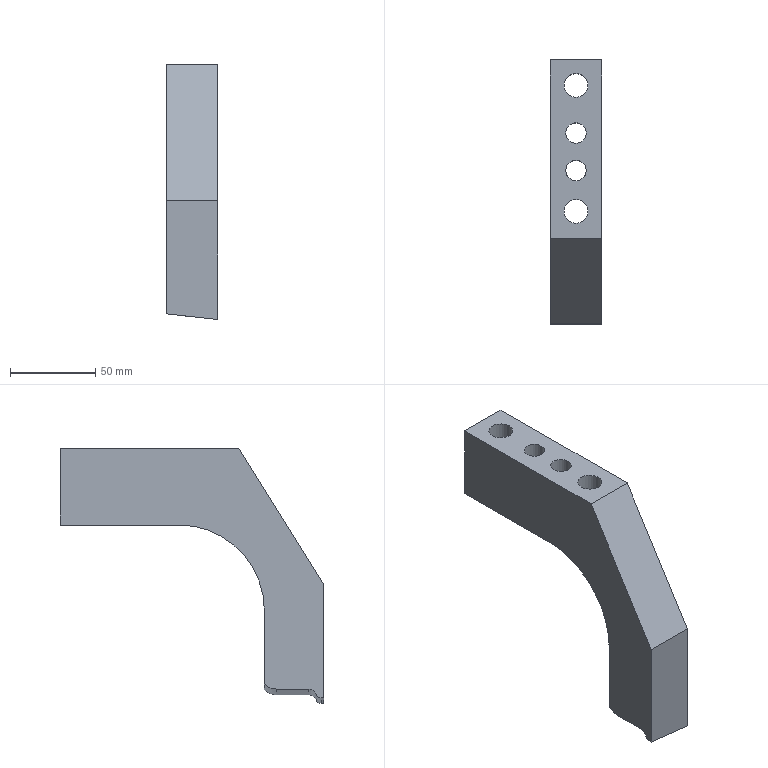Part | NX | features solid 2 | 1 solid | 23 faces | box 30 x 155 x 149.883 mm | volume 237197 mm3 | plane 9 | cylinder 7 | spline 7 | commonest cylinder face diameters 12 x2 14 x2 20 x2 100 x1
STEP:
#1=CARTESIAN_POINT('',(-215.,-438.,-38.417));
#2=VERTEX_POINT('',#1);
#3=CARTESIAN_POINT('',(-185.,-438.,-41.703));
#4=VERTEX_POINT('',#3);
#5=CARTESIAN_POINT('',(-215.,-438.,-38.417));
#6=CARTESIAN_POINT('',(-205.006,-438.,-39.569));
#7=CARTESIAN_POINT('',(-195.006,-438.,-40.665));
#8=CARTESIAN_POINT('',(-185.,-438.,-41.703));
#9=B_SPLINE_CURVE_WITH_KNOTS('',3,(#5,#6,#7,#8),.UNSPECIFIED.,.F.,.F.,(4,4),(0.,0.03018),.UNSPECIFIED.);
#10=EDGE_CURVE('',#2,#4,#9,.T.);
#11=ORIENTED_EDGE('',*,*,#10,.F.);
#12=CARTESIAN_POINT('',(-215.,-438.,5.));
#13=VERTEX_POINT('',#12);
#14=CARTESIAN_POINT('',(-215.,-438.,-220.));
#15=DIRECTION('',(0.,0.,-1.));
#16=VECTOR('',#15,1000.);
#17=LINE('',#14,#16);
#18=EDGE_CURVE('',#13,#2,#17,.T.);
#19=ORIENTED_EDGE('',*,*,#18,.F.);
#20=CARTESIAN_POINT('',(-185.,-438.,5.));
#21=VERTEX_POINT('',#20);
#22=CARTESIAN_POINT('',(-200.,-438.,5.));
#23=DIRECTION('',(-1.,0.,0.));
#24=VECTOR('',#23,1000.);
#25=LINE('',#22,#24);
#26=EDGE_CURVE('',#13,#21,#25,.F.);
#27=ORIENTED_EDGE('',*,*,#26,.T.);
#28=CARTESIAN_POINT('',(-185.,-438.,55.));
#29=DIRECTION('',(0.,0.,-1.));
#30=VECTOR('',#29,1000.);
#31=LINE('',#28,#30);
#32=EDGE_CURVE('',#21,#4,#31,.T.);
#33=ORIENTED_EDGE('',*,*,#32,.T.);
#34=EDGE_LOOP('',(#11,#19,#27,#33));
#35=FACE_BOUND('',#34,.T.);
#36=CARTESIAN_POINT('',(-200.,-438.,17.572));
#37=DIRECTION('',(0.,-1.,0.));
#38=DIRECTION('',(0.,0.,-1.));
#39=AXIS2_PLACEMENT_3D('',#36,#37,#38);
#40=PLANE('',#39);
#41=ADVANCED_FACE('',(#35),#40,.F.);
#42=CARTESIAN_POINT('',(-215.,-473.,20.));
#43=VERTEX_POINT('',#42);
#44=CARTESIAN_POINT('',(-215.,-473.,-46.541));
#45=VERTEX_POINT('',#44);
#46=CARTESIAN_POINT('',(-215.,-473.,-220.));
#47=DIRECTION('',(0.,0.,-1.));
#48=VECTOR('',#47,1000.);
#49=LINE('',#46,#48);
#50=EDGE_CURVE('',#43,#45,#49,.T.);
#51=ORIENTED_EDGE('',*,*,#50,.F.);
#52=CARTESIAN_POINT('',(-215.,-423.,100.));
#53=VERTEX_POINT('',#52);
#54=CARTESIAN_POINT('',(-215.,-423.,100.));
#55=DIRECTION('',(0.,0.53,0.848));
#56=VECTOR('',#55,1000.);
#57=LINE('',#54,#56);
#58=EDGE_CURVE('',#43,#53,#57,.T.);
#59=ORIENTED_EDGE('',*,*,#58,.T.);
#60=CARTESIAN_POINT('',(-215.,-318.,100.));
#61=VERTEX_POINT('',#60);
#62=CARTESIAN_POINT('',(-215.,-449.718,100.));
#63=DIRECTION('',(0.,1.,0.));
#64=VECTOR('',#63,1000.);
#65=LINE('',#62,#64);
#66=EDGE_CURVE('',#53,#61,#65,.T.);
#67=ORIENTED_EDGE('',*,*,#66,.T.);
#68=CARTESIAN_POINT('',(-215.,-318.,55.));
#69=VERTEX_POINT('',#68);
#70=CARTESIAN_POINT('',(-215.,-318.,-220.));
#71=DIRECTION('',(0.,0.,-1.));
#72=VECTOR('',#71,1000.);
#73=LINE('',#70,#72);
#74=EDGE_CURVE('',#61,#69,#73,.T.);
#75=ORIENTED_EDGE('',*,*,#74,.T.);
#76=CARTESIAN_POINT('',(-215.,-388.,55.));
#77=VERTEX_POINT('',#76);
#78=CARTESIAN_POINT('',(-215.,-449.718,55.));
#79=DIRECTION('',(0.,-1.,0.));
#80=VECTOR('',#79,1000.);
#81=LINE('',#78,#80);
#82=EDGE_CURVE('',#69,#77,#81,.T.);
#83=ORIENTED_EDGE('',*,*,#82,.T.);
#84=CARTESIAN_POINT('',(-215.,-388.,5.));
#85=DIRECTION('',(1.,0.,0.));
#86=DIRECTION('',(0.,0.,-1.));
#87=AXIS2_PLACEMENT_3D('',#84,#85,#86);
#88=CIRCLE('',#87,50.);
#89=EDGE_CURVE('',#77,#13,#88,.T.);
#90=ORIENTED_EDGE('',*,*,#89,.T.);
#91=ORIENTED_EDGE('',*,*,#18,.T.);
#92=CARTESIAN_POINT('',(-215.,-445.117,-41.44));
#93=VERTEX_POINT('',#92);
#94=CARTESIAN_POINT('',(-215.,-445.12,-41.44));
#95=CARTESIAN_POINT('',(-215.,-442.447,-41.433));
#96=CARTESIAN_POINT('',(-215.,-439.84,-40.307));
#97=CARTESIAN_POINT('',(-215.,-438.,-38.417));
#98=B_SPLINE_CURVE_WITH_KNOTS('',3,(#94,#95,#96,#97),.UNSPECIFIED.,.F.,.F.,(4,4),(0.,0.007904),.UNSPECIFIED.);
#99=EDGE_CURVE('',#93,#2,#98,.T.);
#100=ORIENTED_EDGE('',*,*,#99,.F.);
#101=CARTESIAN_POINT('',(-215.,-464.023,-41.485));
#102=VERTEX_POINT('',#101);
#103=CARTESIAN_POINT('',(-215.,-445.11,-41.44));
#104=CARTESIAN_POINT('',(-215.,-451.414,-41.455));
#105=CARTESIAN_POINT('',(-215.,-457.718,-41.471));
#106=CARTESIAN_POINT('',(-215.,-464.023,-41.485));
#107=B_SPLINE_CURVE_WITH_KNOTS('',3,(#103,#104,#105,#106),.UNSPECIFIED.,.F.,.F.,(4,4),(0.01573,0.03464),.UNSPECIFIED.);
#108=EDGE_CURVE('',#93,#102,#107,.T.);
#109=ORIENTED_EDGE('',*,*,#108,.T.);
#110=CARTESIAN_POINT('',(-215.,-468.65,-44.642));
#111=VERTEX_POINT('',#110);
#112=CARTESIAN_POINT('',(-215.,-464.023,-41.485));
#113=CARTESIAN_POINT('',(-215.,-466.022,-41.49));
#114=CARTESIAN_POINT('',(-215.,-467.91,-42.787));
#115=CARTESIAN_POINT('',(-215.,-468.65,-44.643));
#116=B_SPLINE_CURVE_WITH_KNOTS('',3,(#112,#113,#114,#115),.UNSPECIFIED.,.F.,.F.,(4,4),(0.,0.005912),.UNSPECIFIED.);
#117=EDGE_CURVE('',#102,#111,#116,.T.);
#118=ORIENTED_EDGE('',*,*,#117,.T.);
#119=CARTESIAN_POINT('',(-215.,-471.426,-46.537));
#120=VERTEX_POINT('',#119);
#121=CARTESIAN_POINT('',(-215.,-471.424,-46.537));
#122=CARTESIAN_POINT('',(-215.,-470.825,-46.534));
#123=CARTESIAN_POINT('',(-215.,-469.586,-46.252));
#124=CARTESIAN_POINT('',(-215.,-468.869,-45.194));
#125=CARTESIAN_POINT('',(-215.,-468.649,-44.64));
#126=B_SPLINE_CURVE_WITH_KNOTS('',3,(#121,#122,#123,#124,#125),.UNSPECIFIED.,.F.,.F.,(4,1,4),(0.001591,0.003375,0.00516),.UNSPECIFIED.);
#127=EDGE_CURVE('',#120,#111,#126,.T.);
#128=ORIENTED_EDGE('',*,*,#127,.F.);
#129=CARTESIAN_POINT('',(-215.,-471.431,-46.537));
#130=CARTESIAN_POINT('',(-215.,-471.954,-46.538));
#131=CARTESIAN_POINT('',(-215.,-472.477,-46.54));
#132=CARTESIAN_POINT('',(-215.,-473.,-46.541));
#133=B_SPLINE_CURVE_WITH_KNOTS('',3,(#129,#130,#131,#132),.UNSPECIFIED.,.F.,.F.,(4,4),(0.005963,0.007533),.UNSPECIFIED.);
#134=EDGE_CURVE('',#120,#45,#133,.T.);
#135=ORIENTED_EDGE('',*,*,#134,.T.);
#136=EDGE_LOOP('',(#51,#59,#67,#75,#83,#90,#91,#100,#109,#118,#128,#135));
#137=FACE_BOUND('',#136,.T.);
#138=CARTESIAN_POINT('',(-215.,-449.718,-220.));
#139=DIRECTION('',(1.,0.,0.));
#140=DIRECTION('',(0.,0.,-1.));
#141=AXIS2_PLACEMENT_3D('',#138,#139,#140);
#142=PLANE('',#141);
#143=ADVANCED_FACE('',(#137),#142,.F.);
#144=CARTESIAN_POINT('',(-185.,-423.,100.));
#145=VERTEX_POINT('',#144);
#146=CARTESIAN_POINT('',(-185.,-318.,100.));
#147=VERTEX_POINT('',#146);
#148=CARTESIAN_POINT('',(-185.,-425.,100.));
#149=DIRECTION('',(0.,1.,0.));
#150=VECTOR('',#149,1000.);
#151=LINE('',#148,#150);
#152=EDGE_CURVE('',#145,#147,#151,.T.);
#153=ORIENTED_EDGE('',*,*,#152,.F.);
#154=CARTESIAN_POINT('',(-185.,-473.,20.));
#155=VERTEX_POINT('',#154);
#156=CARTESIAN_POINT('',(-185.,-443.787,66.742));
#157=DIRECTION('',(0.,-0.53,-0.848));
#158=VECTOR('',#157,1000.);
#159=LINE('',#156,#158);
#160=EDGE_CURVE('',#145,#155,#159,.T.);
#161=ORIENTED_EDGE('',*,*,#160,.T.);
#162=CARTESIAN_POINT('',(-185.,-473.,-49.883));
#163=VERTEX_POINT('',#162);
#164=CARTESIAN_POINT('',(-185.,-473.,55.));
#165=DIRECTION('',(0.,0.,-1.));
#166=VECTOR('',#165,1000.);
#167=LINE('',#164,#166);
#168=EDGE_CURVE('',#155,#163,#167,.T.);
#169=ORIENTED_EDGE('',*,*,#168,.T.);
#170=CARTESIAN_POINT('',(-185.,-471.426,-49.879));
#171=VERTEX_POINT('',#170);
#172=CARTESIAN_POINT('',(-185.,-471.43,-49.88));
#173=CARTESIAN_POINT('',(-185.,-471.953,-49.881));
#174=CARTESIAN_POINT('',(-185.,-472.477,-49.882));
#175=CARTESIAN_POINT('',(-185.,-473.,-49.883));
#176=B_SPLINE_CURVE_WITH_KNOTS('',3,(#172,#173,#174,#175),.UNSPECIFIED.,.F.,.F.,(4,4),(0.005972,0.007542),.UNSPECIFIED.);
#177=EDGE_CURVE('',#171,#163,#176,.T.);
#178=ORIENTED_EDGE('',*,*,#177,.F.);
#179=CARTESIAN_POINT('',(-185.,-468.65,-47.987));
#180=VERTEX_POINT('',#179);
#181=CARTESIAN_POINT('',(-185.,-471.425,-49.879));
#182=CARTESIAN_POINT('',(-185.,-470.826,-49.876));
#183=CARTESIAN_POINT('',(-185.,-469.588,-49.596));
#184=CARTESIAN_POINT('',(-185.,-468.87,-48.54));
#185=CARTESIAN_POINT('',(-185.,-468.649,-47.986));
#186=B_SPLINE_CURVE_WITH_KNOTS('',3,(#181,#182,#183,#184,#185),.UNSPECIFIED.,.F.,.F.,(4,1,4),(0.00159,0.003374,0.005157),.UNSPECIFIED.);
#187=EDGE_CURVE('',#171,#180,#186,.T.);
#188=ORIENTED_EDGE('',*,*,#187,.T.);
#189=CARTESIAN_POINT('',(-185.,-464.023,-44.835));
#190=VERTEX_POINT('',#189);
#191=CARTESIAN_POINT('',(-185.,-464.023,-44.835));
#192=CARTESIAN_POINT('',(-185.,-466.021,-44.839));
#193=CARTESIAN_POINT('',(-185.,-467.91,-46.134));
#194=CARTESIAN_POINT('',(-185.,-468.65,-47.988));
#195=B_SPLINE_CURVE_WITH_KNOTS('',3,(#191,#192,#193,#194),.UNSPECIFIED.,.F.,.F.,(4,4),(0.,0.005909),.UNSPECIFIED.);
#196=EDGE_CURVE('',#190,#180,#195,.T.);
#197=ORIENTED_EDGE('',*,*,#196,.F.);
#198=CARTESIAN_POINT('',(-185.,-445.183,-44.789));
#199=VERTEX_POINT('',#198);
#200=CARTESIAN_POINT('',(-185.,-445.176,-44.789));
#201=CARTESIAN_POINT('',(-185.,-451.458,-44.805));
#202=CARTESIAN_POINT('',(-185.,-457.74,-44.82));
#203=CARTESIAN_POINT('',(-185.,-464.023,-44.835));
#204=B_SPLINE_CURVE_WITH_KNOTS('',3,(#200,#201,#202,#203),.UNSPECIFIED.,.F.,.F.,(4,4),(0.0158,0.03465),.UNSPECIFIED.);
#205=EDGE_CURVE('',#199,#190,#204,.T.);
#206=ORIENTED_EDGE('',*,*,#205,.F.);
#207=CARTESIAN_POINT('',(-185.,-445.185,-44.789));
#208=CARTESIAN_POINT('',(-185.,-442.481,-44.783));
#209=CARTESIAN_POINT('',(-185.,-439.843,-43.631));
#210=CARTESIAN_POINT('',(-185.,-438.,-41.703));
#211=B_SPLINE_CURVE_WITH_KNOTS('',3,(#207,#208,#209,#210),.UNSPECIFIED.,.F.,.F.,(4,4),(0.,0.007995),.UNSPECIFIED.);
#212=EDGE_CURVE('',#199,#4,#211,.T.);
#213=ORIENTED_EDGE('',*,*,#212,.T.);
#214=ORIENTED_EDGE('',*,*,#32,.F.);
#215=CARTESIAN_POINT('',(-185.,-388.,55.));
#216=VERTEX_POINT('',#215);
#217=CARTESIAN_POINT('',(-185.,-388.,5.));
#218=DIRECTION('',(1.,0.,0.));
#219=DIRECTION('',(0.,0.,-1.));
#220=AXIS2_PLACEMENT_3D('',#217,#218,#219);
#221=CIRCLE('',#220,50.);
#222=EDGE_CURVE('',#21,#216,#221,.F.);
#223=ORIENTED_EDGE('',*,*,#222,.T.);
#224=CARTESIAN_POINT('',(-185.,-318.,55.));
#225=VERTEX_POINT('',#224);
#226=CARTESIAN_POINT('',(-185.,-425.,55.));
#227=DIRECTION('',(0.,1.,0.));
#228=VECTOR('',#227,1000.);
#229=LINE('',#226,#228);
#230=EDGE_CURVE('',#216,#225,#229,.T.);
#231=ORIENTED_EDGE('',*,*,#230,.T.);
#232=CARTESIAN_POINT('',(-185.,-318.,55.));
#233=DIRECTION('',(0.,0.,-1.));
#234=VECTOR('',#233,1000.);
#235=LINE('',#232,#234);
#236=EDGE_CURVE('',#147,#225,#235,.T.);
#237=ORIENTED_EDGE('',*,*,#236,.F.);
#238=EDGE_LOOP('',(#153,#161,#169,#178,#188,#197,#206,#213,#214,#223,#231,#237));
#239=FACE_BOUND('',#238,.T.);
#240=CARTESIAN_POINT('',(-185.,-425.,55.));
#241=DIRECTION('',(1.,0.,0.));
#242=DIRECTION('',(0.,0.,-1.));
#243=AXIS2_PLACEMENT_3D('',#240,#241,#242);
#244=PLANE('',#243);
#245=ADVANCED_FACE('',(#239),#244,.T.);
#246=CARTESIAN_POINT('',(-207.,-333.,100.));
#247=VERTEX_POINT('',#246);
#248=CARTESIAN_POINT('',(-200.,-333.,100.));
#249=DIRECTION('',(0.,0.,-1.));
#250=DIRECTION('',(-1.,0.,0.));
#251=AXIS2_PLACEMENT_3D('',#248,#249,#250);
#252=CIRCLE('',#251,7.);
#253=EDGE_CURVE('',#247,#247,#252,.T.);
#254=ORIENTED_EDGE('',*,*,#253,.T.);
#255=EDGE_LOOP('',(#254));
#256=FACE_BOUND('',#255,.T.);
#257=CARTESIAN_POINT('',(-207.,-407.,100.));
#258=VERTEX_POINT('',#257);
#259=CARTESIAN_POINT('',(-200.,-407.,100.));
#260=DIRECTION('',(0.,0.,-1.));
#261=DIRECTION('',(-1.,0.,0.));
#262=AXIS2_PLACEMENT_3D('',#259,#260,#261);
#263=CIRCLE('',#262,7.);
#264=EDGE_CURVE('',#258,#258,#263,.T.);
#265=ORIENTED_EDGE('',*,*,#264,.T.);
#266=EDGE_LOOP('',(#265));
#267=FACE_BOUND('',#266,.T.);
#268=CARTESIAN_POINT('',(-206.,-361.,100.));
#269=VERTEX_POINT('',#268);
#270=CARTESIAN_POINT('',(-200.,-361.,100.));
#271=DIRECTION('',(0.,0.,-1.));
#272=DIRECTION('',(-1.,0.,0.));
#273=AXIS2_PLACEMENT_3D('',#270,#271,#272);
#274=CIRCLE('',#273,6.);
#275=EDGE_CURVE('',#269,#269,#274,.T.);
#276=ORIENTED_EDGE('',*,*,#275,.T.);
#277=EDGE_LOOP('',(#276));
#278=FACE_BOUND('',#277,.T.);
#279=CARTESIAN_POINT('',(-206.,-383.,100.));
#280=VERTEX_POINT('',#279);
#281=CARTESIAN_POINT('',(-200.,-383.,100.));
#282=DIRECTION('',(0.,0.,-1.));
#283=DIRECTION('',(-1.,0.,0.));
#284=AXIS2_PLACEMENT_3D('',#281,#282,#283);
#285=CIRCLE('',#284,6.);
#286=EDGE_CURVE('',#280,#280,#285,.T.);
#287=ORIENTED_EDGE('',*,*,#286,.T.);
#288=EDGE_LOOP('',(#287));
#289=FACE_BOUND('',#288,.T.);
#290=ORIENTED_EDGE('',*,*,#66,.F.);
#291=CARTESIAN_POINT('',(-185.,-423.,100.));
#292=DIRECTION('',(1.,0.,0.));
#293=VECTOR('',#292,1000.);
#294=LINE('',#291,#293);
#295=EDGE_CURVE('',#53,#145,#294,.T.);
#296=ORIENTED_EDGE('',*,*,#295,.T.);
#297=ORIENTED_EDGE('',*,*,#152,.T.);
#298=CARTESIAN_POINT('',(-255.,-318.,100.));
#299=DIRECTION('',(-1.,0.,0.));
#300=VECTOR('',#299,1000.);
#301=LINE('',#298,#300);
#302=EDGE_CURVE('',#147,#61,#301,.T.);
#303=ORIENTED_EDGE('',*,*,#302,.T.);
#304=EDGE_LOOP('',(#290,#296,#297,#303));
#305=FACE_BOUND('',#304,.T.);
#306=CARTESIAN_POINT('',(-255.,-425.,100.));
#307=DIRECTION('',(0.,0.,-1.));
#308=DIRECTION('',(-1.,0.,0.));
#309=AXIS2_PLACEMENT_3D('',#306,#307,#308);
#310=PLANE('',#309);
#311=ADVANCED_FACE('',(#256,#267,#278,#289,#305),#310,.F.);
#312=CARTESIAN_POINT('',(-190.,-333.,75.));
#313=VERTEX_POINT('',#312);
#314=CARTESIAN_POINT('',(-200.,-333.,75.));
#315=DIRECTION('',(0.,0.,-1.));
#316=DIRECTION('',(1.,0.,0.));
#317=AXIS2_PLACEMENT_3D('',#314,#315,#316);
#318=CIRCLE('',#317,10.);
#319=EDGE_CURVE('',#313,#313,#318,.T.);
#320=ORIENTED_EDGE('',*,*,#319,.F.);
#321=EDGE_LOOP('',(#320));
#322=FACE_BOUND('',#321,.T.);
#323=CARTESIAN_POINT('',(-210.,-333.,55.));
#324=VERTEX_POINT('',#323);
#325=CARTESIAN_POINT('',(-200.,-333.,55.));
#326=DIRECTION('',(0.,0.,-1.));
#327=DIRECTION('',(-1.,0.,0.));
#328=AXIS2_PLACEMENT_3D('',#325,#326,#327);
#329=CIRCLE('',#328,10.);
#330=EDGE_CURVE('',#324,#324,#329,.F.);
#331=ORIENTED_EDGE('',*,*,#330,.F.);
#332=EDGE_LOOP('',(#331));
#333=FACE_BOUND('',#332,.T.);
#334=CARTESIAN_POINT('',(-200.,-333.,75.));
#335=DIRECTION('',(0.,0.,-1.));
#336=DIRECTION('',(1.,0.,0.));
#337=AXIS2_PLACEMENT_3D('',#334,#335,#336);
#338=CYLINDRICAL_SURFACE('',#337,10.);
#339=ADVANCED_FACE('',(#322,#333),#338,.F.);
#340=CARTESIAN_POINT('',(-196.683,-397.566,54.076));
#341=VERTEX_POINT('',#340);
#342=CARTESIAN_POINT('',(-203.317,-397.566,54.076));
#343=VERTEX_POINT('',#342);
#344=CARTESIAN_POINT('',(-196.683,-397.566,54.076));
#345=CARTESIAN_POINT('',(-198.827,-396.813,54.223));
#346=CARTESIAN_POINT('',(-201.178,-396.814,54.223));
#347=CARTESIAN_POINT('',(-203.317,-397.566,54.076));
#348=B_SPLINE_CURVE_WITH_KNOTS('',3,(#344,#345,#346,#347),.UNSPECIFIED.,.F.,.F.,(4,4),(0.00252,0.009295),.UNSPECIFIED.);
#349=EDGE_CURVE('',#341,#343,#348,.T.);
#350=ORIENTED_EDGE('',*,*,#349,.F.);
#351=CARTESIAN_POINT('',(-196.683,-397.566,54.076));
#352=CARTESIAN_POINT('',(-194.359,-398.383,53.917));
#353=CARTESIAN_POINT('',(-190.433,-401.807,53.222));
#354=CARTESIAN_POINT('',(-189.595,-407.87,51.002));
#355=CARTESIAN_POINT('',(-191.169,-412.07,48.866));
#356=CARTESIAN_POINT('',(-193.31,-414.69,47.309));
#357=CARTESIAN_POINT('',(-196.321,-416.532,46.069));
#358=CARTESIAN_POINT('',(-200.012,-417.236,45.56));
#359=CARTESIAN_POINT('',(-203.706,-416.522,46.076));
#360=CARTESIAN_POINT('',(-207.707,-414.057,47.736));
#361=CARTESIAN_POINT('',(-210.569,-409.042,50.578));
#362=CARTESIAN_POINT('',(-209.564,-401.814,53.218));
#363=CARTESIAN_POINT('',(-205.645,-398.384,53.917));
#364=CARTESIAN_POINT('',(-203.317,-397.566,54.076));
#365=B_SPLINE_CURVE_WITH_KNOTS('',3,(#351,#352,#353,#354,#355,#356,#357,#358,#359,#360,#361,#362,#363,#364),.UNSPECIFIED.,.F.,.F.,(4,1,1,1,1,1,1,1,1,1,1,4),(0.03954,0.04689,0.05424,0.05791,0.06159,0.06526,0.06894,0.07261,0.07629,0.08363,0.09098,0.09833),.UNSPECIFIED.);
#366=EDGE_CURVE('',#341,#343,#365,.T.);
#367=ORIENTED_EDGE('',*,*,#366,.T.);
#368=EDGE_LOOP('',(#350,#367));
#369=FACE_BOUND('',#368,.T.);
#370=CARTESIAN_POINT('',(-190.,-407.,75.));
#371=VERTEX_POINT('',#370);
#372=CARTESIAN_POINT('',(-200.,-407.,75.));
#373=DIRECTION('',(0.,0.,-1.));
#374=DIRECTION('',(1.,0.,0.));
#375=AXIS2_PLACEMENT_3D('',#372,#373,#374);
#376=CIRCLE('',#375,10.);
#377=EDGE_CURVE('',#371,#371,#376,.T.);
#378=ORIENTED_EDGE('',*,*,#377,.F.);
#379=EDGE_LOOP('',(#378));
#380=FACE_BOUND('',#379,.T.);
#381=CARTESIAN_POINT('',(-200.,-407.,75.));
#382=DIRECTION('',(0.,0.,-1.));
#383=DIRECTION('',(1.,0.,0.));
#384=AXIS2_PLACEMENT_3D('',#381,#382,#383);
#385=CYLINDRICAL_SURFACE('',#384,10.);
#386=ADVANCED_FACE('',(#369,#380),#385,.F.);
#387=ORIENTED_EDGE('',*,*,#275,.F.);
#388=EDGE_LOOP('',(#387));
#389=FACE_BOUND('',#388,.T.);
#390=CARTESIAN_POINT('',(-206.,-361.,55.));
#391=VERTEX_POINT('',#390);
#392=CARTESIAN_POINT('',(-200.,-361.,55.));
#393=DIRECTION('',(0.,0.,-1.));
#394=DIRECTION('',(-1.,0.,0.));
#395=AXIS2_PLACEMENT_3D('',#392,#393,#394);
#396=CIRCLE('',#395,6.);
#397=EDGE_CURVE('',#391,#391,#396,.T.);
#398=ORIENTED_EDGE('',*,*,#397,.T.);
#399=EDGE_LOOP('',(#398));
#400=FACE_BOUND('',#399,.T.);
#401=CARTESIAN_POINT('',(-200.,-361.,105.));
#402=DIRECTION('',(0.,0.,-1.));
#403=DIRECTION('',(-1.,0.,0.));
#404=AXIS2_PLACEMENT_3D('',#401,#402,#403);
#405=CYLINDRICAL_SURFACE('',#404,6.);
#406=ADVANCED_FACE('',(#389,#400),#405,.F.);
#407=ORIENTED_EDGE('',*,*,#286,.F.);
#408=EDGE_LOOP('',(#407));
#409=FACE_BOUND('',#408,.T.);
#410=CARTESIAN_POINT('',(-196.683,-388.,55.));
#411=VERTEX_POINT('',#410);
#412=CARTESIAN_POINT('',(-203.317,-388.,55.));
#413=VERTEX_POINT('',#412);
#414=CARTESIAN_POINT('',(-200.,-383.,55.));
#415=DIRECTION('',(0.,0.,-1.));
#416=DIRECTION('',(-1.,0.,0.));
#417=AXIS2_PLACEMENT_3D('',#414,#415,#416);
#418=CIRCLE('',#417,6.);
#419=EDGE_CURVE('',#411,#413,#418,.T.);
#420=ORIENTED_EDGE('',*,*,#419,.T.);
#421=CARTESIAN_POINT('',(-200.,-383.,55.));
#422=DIRECTION('',(0.,0.,-1.));
#423=DIRECTION('',(-1.,0.,0.));
#424=AXIS2_PLACEMENT_3D('',#421,#422,#423);
#425=CIRCLE('',#424,6.);
#426=EDGE_CURVE('',#413,#411,#425,.T.);
#427=ORIENTED_EDGE('',*,*,#426,.T.);
#428=EDGE_LOOP('',(#420,#427));
#429=FACE_BOUND('',#428,.T.);
#430=CARTESIAN_POINT('',(-200.,-383.,105.));
#431=DIRECTION('',(0.,0.,-1.));
#432=DIRECTION('',(-1.,0.,0.));
#433=AXIS2_PLACEMENT_3D('',#430,#431,#432);
#434=CYLINDRICAL_SURFACE('',#433,6.);
#435=ADVANCED_FACE('',(#409,#429),#434,.F.);
#436=CARTESIAN_POINT('',(-193.,-333.,75.));
#437=VERTEX_POINT('',#436);
#438=CARTESIAN_POINT('',(-200.,-333.,75.));
#439=DIRECTION('',(0.,0.,1.));
#440=DIRECTION('',(1.,0.,0.));
#441=AXIS2_PLACEMENT_3D('',#438,#439,#440);
#442=CIRCLE('',#441,7.);
#443=EDGE_CURVE('',#437,#437,#442,.T.);
#444=ORIENTED_EDGE('',*,*,#443,.F.);
#445=EDGE_LOOP('',(#444));
#446=FACE_BOUND('',#445,.T.);
#447=ORIENTED_EDGE('',*,*,#253,.F.);
#448=EDGE_LOOP('',(#447));
#449=FACE_BOUND('',#448,.T.);
#450=CARTESIAN_POINT('',(-200.,-333.,75.));
#451=DIRECTION('',(0.,0.,1.));
#452=DIRECTION('',(-1.,0.,0.));
#453=AXIS2_PLACEMENT_3D('',#450,#451,#452);
#454=CYLINDRICAL_SURFACE('',#453,7.);
#455=ADVANCED_FACE('',(#446,#449),#454,.F.);
#456=ORIENTED_EDGE('',*,*,#443,.T.);
#457=EDGE_LOOP('',(#456));
#458=FACE_BOUND('',#457,.T.);
#459=ORIENTED_EDGE('',*,*,#319,.T.);
#460=EDGE_LOOP('',(#459));
#461=FACE_BOUND('',#460,.T.);
#462=CARTESIAN_POINT('',(-200.,-333.,75.));
#463=DIRECTION('',(0.,0.,1.));
#464=DIRECTION('',(-1.,0.,0.));
#465=AXIS2_PLACEMENT_3D('',#462,#463,#464);
#466=PLANE('',#465);
#467=ADVANCED_FACE('',(#458,#461),#466,.F.);
#468=CARTESIAN_POINT('',(-193.,-407.,75.));
#469=VERTEX_POINT('',#468);
#470=CARTESIAN_POINT('',(-200.,-407.,75.));
#471=DIRECTION('',(0.,0.,1.));
#472=DIRECTION('',(1.,0.,0.));
#473=AXIS2_PLACEMENT_3D('',#470,#471,#472);
#474=CIRCLE('',#473,7.);
#475=EDGE_CURVE('',#469,#469,#474,.T.);
#476=ORIENTED_EDGE('',*,*,#475,.F.);
#477=EDGE_LOOP('',(#476));
#478=FACE_BOUND('',#477,.T.);
#479=ORIENTED_EDGE('',*,*,#264,.F.);
#480=EDGE_LOOP('',(#479));
#481=FACE_BOUND('',#480,.T.);
#482=CARTESIAN_POINT('',(-200.,-407.,75.));
#483=DIRECTION('',(0.,0.,1.));
#484=DIRECTION('',(-1.,0.,0.));
#485=AXIS2_PLACEMENT_3D('',#482,#483,#484);
#486=CYLINDRICAL_SURFACE('',#485,7.);
#487=ADVANCED_FACE('',(#478,#481),#486,.F.);
#488=ORIENTED_EDGE('',*,*,#475,.T.);
#489=EDGE_LOOP('',(#488));
#490=FACE_BOUND('',#489,.T.);
#491=ORIENTED_EDGE('',*,*,#377,.T.);
#492=EDGE_LOOP('',(#491));
#493=FACE_BOUND('',#492,.T.);
#494=CARTESIAN_POINT('',(-200.,-402.,75.));
#495=DIRECTION('',(0.,0.,1.));
#496=DIRECTION('',(-1.,0.,0.));
#497=AXIS2_PLACEMENT_3D('',#494,#495,#496);
#498=PLANE('',#497);
#499=ADVANCED_FACE('',(#490,#493),#498,.F.);
#500=ORIENTED_EDGE('',*,*,#230,.F.);
#501=CARTESIAN_POINT('',(-185.,-388.,55.));
#502=DIRECTION('',(-1.,0.,0.));
#503=VECTOR('',#502,1000.);
#504=LINE('',#501,#503);
#505=EDGE_CURVE('',#216,#411,#504,.T.);
#506=ORIENTED_EDGE('',*,*,#505,.T.);
#507=ORIENTED_EDGE('',*,*,#426,.F.);
#508=CARTESIAN_POINT('',(-185.,-388.,55.));
#509=DIRECTION('',(-1.,0.,0.));
#510=VECTOR('',#509,1000.);
#511=LINE('',#508,#510);
#512=EDGE_CURVE('',#413,#77,#511,.T.);
#513=ORIENTED_EDGE('',*,*,#512,.T.);
#514=ORIENTED_EDGE('',*,*,#82,.F.);
#515=CARTESIAN_POINT('',(-185.,-318.,55.));
#516=DIRECTION('',(-1.,0.,0.));
#517=VECTOR('',#516,1000.);
#518=LINE('',#515,#517);
#519=EDGE_CURVE('',#225,#69,#518,.T.);
#520=ORIENTED_EDGE('',*,*,#519,.F.);
#521=EDGE_LOOP('',(#500,#506,#507,#513,#514,#520));
#522=FACE_BOUND('',#521,.T.);
#523=ORIENTED_EDGE('',*,*,#397,.F.);
#524=EDGE_LOOP('',(#523));
#525=FACE_BOUND('',#524,.T.);
#526=ORIENTED_EDGE('',*,*,#330,.T.);
#527=EDGE_LOOP('',(#526));
#528=FACE_BOUND('',#527,.T.);
#529=CARTESIAN_POINT('',(-185.,-410.,55.));
#530=DIRECTION('',(0.,0.,-1.));
#531=DIRECTION('',(-1.,0.,0.));
#532=AXIS2_PLACEMENT_3D('',#529,#530,#531);
#533=PLANE('',#532);
#534=ADVANCED_FACE('',(#522,#525,#528),#533,.T.);
#535=ORIENTED_EDGE('',*,*,#236,.T.);
#536=ORIENTED_EDGE('',*,*,#519,.T.);
#537=ORIENTED_EDGE('',*,*,#74,.F.);
#538=ORIENTED_EDGE('',*,*,#302,.F.);
#539=EDGE_LOOP('',(#535,#536,#537,#538));
#540=FACE_BOUND('',#539,.T.);
#541=CARTESIAN_POINT('',(-215.,-318.,100.));
#542=CARTESIAN_POINT('',(-185.,-318.,100.));
#543=CARTESIAN_POINT('',(-215.,-318.,55.));
#544=CARTESIAN_POINT('',(-185.,-318.,55.));
#545=B_SPLINE_SURFACE_WITH_KNOTS('',1,1,((#541,#542),(#543,#544)),.PLANE_SURF.,.F.,.F.,.F.,(2,2),(2,2),(0.3333,0.4238),(0.3333,0.6667),.PIECEWISE_BEZIER_KNOTS.);
#546=ADVANCED_FACE('',(#540),#545,.F.);
#547=ORIENTED_EDGE('',*,*,#168,.F.);
#548=CARTESIAN_POINT('',(-215.,-473.,20.));
#549=DIRECTION('',(-1.,0.,0.));
#550=VECTOR('',#549,1000.);
#551=LINE('',#548,#550);
#552=EDGE_CURVE('',#155,#43,#551,.T.);
#553=ORIENTED_EDGE('',*,*,#552,.T.);
#554=ORIENTED_EDGE('',*,*,#50,.T.);
#555=CARTESIAN_POINT('',(-185.,-473.,-49.883));
#556=CARTESIAN_POINT('',(-195.007,-473.,-48.83));
#557=CARTESIAN_POINT('',(-205.007,-473.,-47.715));
#558=CARTESIAN_POINT('',(-215.,-473.,-46.541));
#559=B_SPLINE_CURVE_WITH_KNOTS('',3,(#555,#556,#557,#558),.UNSPECIFIED.,.F.,.F.,(4,4),(0.,0.03019),.UNSPECIFIED.);
#560=EDGE_CURVE('',#163,#45,#559,.T.);
#561=ORIENTED_EDGE('',*,*,#560,.F.);
#562=EDGE_LOOP('',(#547,#553,#554,#561));
#563=FACE_BOUND('',#562,.T.);
#564=CARTESIAN_POINT('',(-1500.,-473.,0.));
#565=DIRECTION('',(0.,-1.,0.));
#566=DIRECTION('',(0.,0.,-1.));
#567=AXIS2_PLACEMENT_3D('',#564,#565,#566);
#568=PLANE('',#567);
#569=ADVANCED_FACE('',(#563),#568,.T.);
#570=CARTESIAN_POINT('',(-196.683,-388.,5.));
#571=DIRECTION('',(1.,0.,0.));
#572=DIRECTION('',(0.,0.,-1.));
#573=AXIS2_PLACEMENT_3D('',#570,#571,#572);
#574=CIRCLE('',#573,50.);
#575=EDGE_CURVE('',#341,#411,#574,.F.);
#576=ORIENTED_EDGE('',*,*,#575,.F.);
#577=ORIENTED_EDGE('',*,*,#349,.T.);
#578=CARTESIAN_POINT('',(-203.317,-388.,5.));
#579=DIRECTION('',(-1.,0.,0.));
#580=DIRECTION('',(0.,0.,1.));
#581=AXIS2_PLACEMENT_3D('',#578,#579,#580);
#582=CIRCLE('',#581,50.);
#583=EDGE_CURVE('',#413,#343,#582,.F.);
#584=ORIENTED_EDGE('',*,*,#583,.F.);
#585=ORIENTED_EDGE('',*,*,#419,.F.);
#586=EDGE_LOOP('',(#576,#577,#584,#585));
#587=FACE_BOUND('',#586,.T.);
#588=CARTESIAN_POINT('',(-196.683,-388.,55.));
#589=CARTESIAN_POINT('',(-196.683,-392.857,55.));
#590=CARTESIAN_POINT('',(-196.683,-397.623,54.065));
#591=CARTESIAN_POINT('',(-197.067,-388.255,55.));
#592=CARTESIAN_POINT('',(-197.067,-393.098,54.975));
#593=CARTESIAN_POINT('',(-197.07,-397.846,54.022));
#594=CARTESIAN_POINT('',(-198.019,-388.763,55.));
#595=CARTESIAN_POINT('',(-198.019,-393.578,54.926));
#596=CARTESIAN_POINT('',(-198.025,-398.291,53.935));
#597=CARTESIAN_POINT('',(-200.,-389.119,55.));
#598=CARTESIAN_POINT('',(-200.,-393.914,54.893));
#599=CARTESIAN_POINT('',(-200.,-398.602,53.876));
#600=CARTESIAN_POINT('',(-201.981,-388.763,55.));
#601=CARTESIAN_POINT('',(-201.981,-393.578,54.926));
#602=CARTESIAN_POINT('',(-201.974,-398.291,53.935));
#603=CARTESIAN_POINT('',(-202.933,-388.255,55.));
#604=CARTESIAN_POINT('',(-202.933,-393.098,54.975));
#605=CARTESIAN_POINT('',(-202.93,-397.846,54.022));
#606=CARTESIAN_POINT('',(-203.317,-388.,55.));
#607=CARTESIAN_POINT('',(-203.317,-392.857,55.));
#608=CARTESIAN_POINT('',(-203.317,-397.623,54.065));
#609=(BOUNDED_SURFACE()B_SPLINE_SURFACE(3,2,((#588,#589,#590),(#591,#592,#593),(#594,#595,#596),(#597,#598,#599),(#600,#601,#602),(#603,#604,#605),(#606,#607,#608)),.UNSPECIFIED.,.F.,.F.,.F.)B_SPLINE_SURFACE_WITH_KNOTS((4,1,1,1,4),(3,3),(0.08051,0.08216,0.0838,0.08545,0.0871),(0.,0.1321),.UNSPECIFIED.)GEOMETRIC_REPRESENTATION_ITEM()RATIONAL_B_SPLINE_SURFACE(((1.,0.9613,0.9329),(1.,0.9616,0.9333),(1.,0.962,0.9341),(1.,0.9624,0.9347),(1.,0.962,0.9341),(1.,0.9616,0.9333),(1.,0.9613,0.9329)))REPRESENTATION_ITEM('')SURFACE());
#610=ADVANCED_FACE('',(#587),#609,.F.);
#611=ORIENTED_EDGE('',*,*,#222,.F.);
#612=ORIENTED_EDGE('',*,*,#26,.F.);
#613=ORIENTED_EDGE('',*,*,#89,.F.);
#614=ORIENTED_EDGE('',*,*,#512,.F.);
#615=ORIENTED_EDGE('',*,*,#583,.T.);
#616=ORIENTED_EDGE('',*,*,#366,.F.);
#617=ORIENTED_EDGE('',*,*,#575,.T.);
#618=ORIENTED_EDGE('',*,*,#505,.F.);
#619=EDGE_LOOP('',(#611,#612,#613,#614,#615,#616,#617,#618));
#620=FACE_BOUND('',#619,.T.);
#621=CARTESIAN_POINT('',(-185.,-388.,5.));
#622=DIRECTION('',(-1.,0.,0.));
#623=DIRECTION('',(0.,0.,1.));
#624=AXIS2_PLACEMENT_3D('',#621,#622,#623);
#625=CYLINDRICAL_SURFACE('',#624,50.);
#626=ADVANCED_FACE('',(#620),#625,.F.);
#627=ORIENTED_EDGE('',*,*,#127,.T.);
#628=CARTESIAN_POINT('',(-215.,-468.649,-44.64));
#629=CARTESIAN_POINT('',(-204.953,-468.649,-45.821));
#630=CARTESIAN_POINT('',(-194.953,-468.649,-46.937));
#631=CARTESIAN_POINT('',(-185.,-468.649,-47.986));
#632=B_SPLINE_CURVE_WITH_KNOTS('',3,(#628,#629,#630,#631),.UNSPECIFIED.,.F.,.F.,(4,4),(0.7825,0.8381),.UNSPECIFIED.);
#633=EDGE_CURVE('',#111,#180,#632,.T.);
#634=ORIENTED_EDGE('',*,*,#633,.T.);
#635=ORIENTED_EDGE('',*,*,#187,.F.);
#636=CARTESIAN_POINT('',(-185.,-471.425,-49.879));
#637=CARTESIAN_POINT('',(-194.953,-471.425,-48.831));
#638=CARTESIAN_POINT('',(-204.953,-471.424,-47.717));
#639=CARTESIAN_POINT('',(-215.,-471.424,-46.537));
#640=B_SPLINE_CURVE_WITH_KNOTS('',3,(#636,#637,#638,#639),.UNSPECIFIED.,.F.,.F.,(4,4),(0.1617,0.2174),.UNSPECIFIED.);
#641=EDGE_CURVE('',#171,#120,#640,.T.);
#642=ORIENTED_EDGE('',*,*,#641,.T.);
#643=EDGE_LOOP('',(#627,#634,#635,#642));
#644=FACE_BOUND('',#643,.T.);
#645=CARTESIAN_POINT('',(-184.799,-472.798,-49.73));
#646=CARTESIAN_POINT('',(-184.828,-471.841,-49.949));
#647=CARTESIAN_POINT('',(-184.83,-471.011,-49.99));
#648=CARTESIAN_POINT('',(-184.804,-470.308,-49.853));
#649=CARTESIAN_POINT('',(-184.732,-469.535,-49.433));
#650=CARTESIAN_POINT('',(-184.612,-468.983,-48.706));
#651=CARTESIAN_POINT('',(-184.578,-468.857,-48.5));
#652=CARTESIAN_POINT('',(-184.541,-468.744,-48.275));
#653=CARTESIAN_POINT('',(-184.501,-468.646,-48.03));
#654=CARTESIAN_POINT('',(-190.951,-472.469,-49.159));
#655=CARTESIAN_POINT('',(-190.973,-471.547,-49.329));
#656=CARTESIAN_POINT('',(-190.967,-470.752,-49.321));
#657=CARTESIAN_POINT('',(-190.934,-470.084,-49.136));
#658=CARTESIAN_POINT('',(-190.851,-469.358,-48.651));
#659=CARTESIAN_POINT('',(-190.721,-468.851,-47.861));
#660=CARTESIAN_POINT('',(-190.685,-468.736,-47.64));
#661=CARTESIAN_POINT('',(-190.645,-468.634,-47.399));
#662=CARTESIAN_POINT('',(-190.603,-468.547,-47.138));
#663=CARTESIAN_POINT('',(-197.096,-472.172,-48.544));
#664=CARTESIAN_POINT('',(-197.111,-471.282,-48.668));
#665=CARTESIAN_POINT('',(-197.098,-470.521,-48.614));
#666=CARTESIAN_POINT('',(-197.057,-469.887,-48.382));
#667=CARTESIAN_POINT('',(-196.965,-469.204,-47.837));
#668=CARTESIAN_POINT('',(-196.826,-468.739,-46.988));
#669=CARTESIAN_POINT('',(-196.787,-468.635,-46.751));
#670=CARTESIAN_POINT('',(-196.745,-468.544,-46.495));
#671=CARTESIAN_POINT('',(-196.7,-468.468,-46.22));
#672=CARTESIAN_POINT('',(-203.235,-471.902,-47.89));
#673=CARTESIAN_POINT('',(-203.243,-471.045,-47.969));
#674=CARTESIAN_POINT('',(-203.223,-470.315,-47.871));
#675=CARTESIAN_POINT('',(-203.176,-469.712,-47.597));
#676=CARTESIAN_POINT('',(-203.075,-469.07,-46.994));
#677=CARTESIAN_POINT('',(-202.927,-468.645,-46.089));
#678=CARTESIAN_POINT('',(-202.886,-468.551,-45.839));
#679=CARTESIAN_POINT('',(-202.842,-468.471,-45.569));
#680=CARTESIAN_POINT('',(-202.795,-468.404,-45.279));
#681=CARTESIAN_POINT('',(-209.369,-471.659,-47.2));
#682=CARTESIAN_POINT('',(-209.37,-470.831,-47.238));
#683=CARTESIAN_POINT('',(-209.344,-470.131,-47.099));
#684=CARTESIAN_POINT('',(-209.29,-469.557,-46.783));
#685=CARTESIAN_POINT('',(-209.18,-468.954,-46.127));
#686=CARTESIAN_POINT('',(-209.024,-468.567,-45.17));
#687=CARTESIAN_POINT('',(-208.981,-468.482,-44.906));
#688=CARTESIAN_POINT('',(-208.935,-468.411,-44.622));
#689=CARTESIAN_POINT('',(-208.886,-468.354,-44.32));
#690=CARTESIAN_POINT('',(-215.497,-471.438,-46.479));
#691=CARTESIAN_POINT('',(-215.493,-470.638,-46.477));
#692=CARTESIAN_POINT('',(-215.46,-469.966,-46.299));
#693=CARTESIAN_POINT('',(-215.4,-469.42,-45.945));
#694=CARTESIAN_POINT('',(-215.283,-468.852,-45.238));
#695=CARTESIAN_POINT('',(-215.119,-468.501,-44.232));
#696=CARTESIAN_POINT('',(-215.074,-468.425,-43.955));
#697=CARTESIAN_POINT('',(-215.026,-468.363,-43.66));
#698=CARTESIAN_POINT('',(-214.974,-468.315,-43.344));
#699=B_SPLINE_SURFACE_WITH_KNOTS('',5,5,((#645,#646,#647,#648,#649,#650,#651,#652,#653),(#654,#655,#656,#657,#658,#659,#660,#661,#662),(#663,#664,#665,#666,#667,#668,#669,#670,#671),(#672,#673,#674,#675,#676,#677,#678,#679,#680),(#681,#682,#683,#684,#685,#686,#687,#688,#689),(#690,#691,#692,#693,#694,#695,#696,#697,#698)),.UNSPECIFIED.,.F.,.F.,.F.,(6,6),(6,3,6),(0.1524,0.2052),(0.2588,0.486,0.5639),.UNSPECIFIED.);
#700=ADVANCED_FACE('',(#644),#699,.T.);
#701=CARTESIAN_POINT('',(-185.,-464.023,-44.835));
#702=CARTESIAN_POINT('',(-195.003,-464.023,-43.779));
#703=CARTESIAN_POINT('',(-205.003,-464.023,-42.662));
#704=CARTESIAN_POINT('',(-215.,-464.023,-41.485));
#705=B_SPLINE_CURVE_WITH_KNOTS('',3,(#701,#702,#703,#704),.UNSPECIFIED.,.F.,.F.,(4,4),(0.165,0.2227),.UNSPECIFIED.);
#706=EDGE_CURVE('',#190,#102,#705,.T.);
#707=ORIENTED_EDGE('',*,*,#706,.F.);
#708=ORIENTED_EDGE('',*,*,#196,.T.);
#709=ORIENTED_EDGE('',*,*,#633,.F.);
#710=ORIENTED_EDGE('',*,*,#117,.F.);
#711=EDGE_LOOP('',(#707,#708,#709,#710));
#712=FACE_BOUND('',#711,.T.);
#713=CARTESIAN_POINT('',(-184.489,-464.023,-44.888));
#714=CARTESIAN_POINT('',(-184.49,-465.209,-44.891));
#715=CARTESIAN_POINT('',(-184.527,-466.395,-45.244));
#716=CARTESIAN_POINT('',(-184.601,-467.439,-45.948));
#717=CARTESIAN_POINT('',(-184.702,-468.208,-46.912));
#718=CARTESIAN_POINT('',(-184.818,-468.65,-48.007));
#719=CARTESIAN_POINT('',(-190.63,-464.023,-44.242));
#720=CARTESIAN_POINT('',(-190.63,-465.209,-44.245));
#721=CARTESIAN_POINT('',(-190.668,-466.395,-44.597));
#722=CARTESIAN_POINT('',(-190.744,-467.439,-45.301));
#723=CARTESIAN_POINT('',(-190.848,-468.208,-46.265));
#724=CARTESIAN_POINT('',(-190.966,-468.65,-47.36));
#725=CARTESIAN_POINT('',(-196.769,-464.023,-43.576));
#726=CARTESIAN_POINT('',(-196.769,-465.209,-43.579));
#727=CARTESIAN_POINT('',(-196.808,-466.395,-43.931));
#728=CARTESIAN_POINT('',(-196.886,-467.439,-44.635));
#729=CARTESIAN_POINT('',(-196.992,-468.208,-45.599));
#730=CARTESIAN_POINT('',(-197.113,-468.65,-46.693));
#731=CARTESIAN_POINT('',(-202.907,-464.023,-42.891));
#732=CARTESIAN_POINT('',(-202.908,-465.209,-42.894));
#733=CARTESIAN_POINT('',(-202.947,-466.395,-43.246));
#734=CARTESIAN_POINT('',(-203.027,-467.439,-43.949));
#735=CARTESIAN_POINT('',(-203.136,-468.208,-44.913));
#736=CARTESIAN_POINT('',(-203.259,-468.65,-46.007));
#737=CARTESIAN_POINT('',(-209.045,-464.023,-42.187));
#738=CARTESIAN_POINT('',(-209.045,-465.209,-42.19));
#739=CARTESIAN_POINT('',(-209.086,-466.395,-42.542));
#740=CARTESIAN_POINT('',(-209.167,-467.439,-43.245));
#741=CARTESIAN_POINT('',(-209.278,-468.208,-44.208));
#742=CARTESIAN_POINT('',(-209.404,-468.65,-45.302));
#743=CARTESIAN_POINT('',(-215.182,-464.023,-41.464));
#744=CARTESIAN_POINT('',(-215.182,-465.209,-41.467));
#745=CARTESIAN_POINT('',(-215.224,-466.395,-41.819));
#746=CARTESIAN_POINT('',(-215.307,-467.439,-42.522));
#747=CARTESIAN_POINT('',(-215.42,-468.208,-43.485));
#748=CARTESIAN_POINT('',(-215.549,-468.65,-44.578));
#749=B_SPLINE_SURFACE_WITH_KNOTS('',5,5,((#713,#714,#715,#716,#717,#718),(#719,#720,#721,#722,#723,#724),(#725,#726,#727,#728,#729,#730),(#731,#732,#733,#734,#735,#736),(#737,#738,#739,#740,#741,#742),(#743,#744,#745,#746,#747,#748)),.UNSPECIFIED.,.F.,.F.,.F.,(6,6),(6,6),(0.1497,0.2036),(0.,0.994),.PIECEWISE_BEZIER_KNOTS.);
#750=ADVANCED_FACE('',(#712),#749,.F.);
#751=CARTESIAN_POINT('',(-215.,-445.11,-41.44));
#752=CARTESIAN_POINT('',(-205.265,-445.134,-42.586));
#753=CARTESIAN_POINT('',(-195.265,-445.156,-43.706));
#754=CARTESIAN_POINT('',(-185.,-445.176,-44.789));
#755=B_SPLINE_CURVE_WITH_KNOTS('',3,(#751,#752,#753,#754),.UNSPECIFIED.,.F.,.F.,(4,4),(0.7963,0.8527),.UNSPECIFIED.);
#756=EDGE_CURVE('',#93,#199,#755,.T.);
#757=ORIENTED_EDGE('',*,*,#756,.T.);
#758=ORIENTED_EDGE('',*,*,#205,.T.);
#759=ORIENTED_EDGE('',*,*,#706,.T.);
#760=ORIENTED_EDGE('',*,*,#108,.F.);
#761=EDGE_LOOP('',(#757,#758,#759,#760));
#762=FACE_BOUND('',#761,.T.);
#763=CARTESIAN_POINT('',(-215.,-444.996,-41.44));
#764=CARTESIAN_POINT('',(-215.,-451.349,-41.455));
#765=CARTESIAN_POINT('',(-215.,-457.701,-41.471));
#766=CARTESIAN_POINT('',(-215.,-464.053,-41.486));
#767=CARTESIAN_POINT('',(-208.964,-444.994,-42.15));
#768=CARTESIAN_POINT('',(-208.964,-451.347,-42.166));
#769=CARTESIAN_POINT('',(-208.964,-457.699,-42.181));
#770=CARTESIAN_POINT('',(-208.964,-464.051,-42.196));
#771=CARTESIAN_POINT('',(-202.928,-444.992,-42.842));
#772=CARTESIAN_POINT('',(-202.928,-451.345,-42.858));
#773=CARTESIAN_POINT('',(-202.928,-457.697,-42.873));
#774=CARTESIAN_POINT('',(-202.928,-464.049,-42.888));
#775=CARTESIAN_POINT('',(-196.892,-444.99,-43.516));
#776=CARTESIAN_POINT('',(-196.892,-451.343,-43.532));
#777=CARTESIAN_POINT('',(-196.892,-457.695,-43.547));
#778=CARTESIAN_POINT('',(-196.892,-464.047,-43.562));
#779=CARTESIAN_POINT('',(-190.856,-444.988,-44.171));
#780=CARTESIAN_POINT('',(-190.856,-451.341,-44.187));
#781=CARTESIAN_POINT('',(-190.856,-457.693,-44.202));
#782=CARTESIAN_POINT('',(-190.856,-464.046,-44.217));
#783=CARTESIAN_POINT('',(-184.82,-444.986,-44.808));
#784=CARTESIAN_POINT('',(-184.82,-451.339,-44.823));
#785=CARTESIAN_POINT('',(-184.82,-457.691,-44.839));
#786=CARTESIAN_POINT('',(-184.82,-464.044,-44.854));
#787=B_SPLINE_SURFACE_WITH_KNOTS('',5,3,((#763,#764,#765,#766),(#767,#768,#769,#770),(#771,#772,#773,#774),(#775,#776,#777,#778),(#779,#780,#781,#782),(#783,#784,#785,#786)),.UNSPECIFIED.,.F.,.F.,.F.,(6,6),(4,4),(0.7887,0.8437),(0.4503,1.),.PIECEWISE_BEZIER_KNOTS.);
#788=ADVANCED_FACE('',(#762),#787,.T.);
#789=ORIENTED_EDGE('',*,*,#641,.F.);
#790=ORIENTED_EDGE('',*,*,#177,.T.);
#791=ORIENTED_EDGE('',*,*,#560,.T.);
#792=ORIENTED_EDGE('',*,*,#134,.F.);
#793=EDGE_LOOP('',(#789,#790,#791,#792));
#794=FACE_BOUND('',#793,.T.);
#795=CARTESIAN_POINT('',(-185.,-471.412,-49.88));
#796=CARTESIAN_POINT('',(-185.,-471.945,-49.881));
#797=CARTESIAN_POINT('',(-185.,-472.477,-49.882));
#798=CARTESIAN_POINT('',(-185.,-473.009,-49.883));
#799=CARTESIAN_POINT('',(-191.036,-471.414,-49.244));
#800=CARTESIAN_POINT('',(-191.036,-471.946,-49.245));
#801=CARTESIAN_POINT('',(-191.036,-472.479,-49.246));
#802=CARTESIAN_POINT('',(-191.036,-473.011,-49.248));
#803=CARTESIAN_POINT('',(-197.072,-471.416,-48.59));
#804=CARTESIAN_POINT('',(-197.072,-471.948,-48.591));
#805=CARTESIAN_POINT('',(-197.072,-472.481,-48.592));
#806=CARTESIAN_POINT('',(-197.072,-473.013,-48.593));
#807=CARTESIAN_POINT('',(-203.108,-471.418,-47.917));
#808=CARTESIAN_POINT('',(-203.108,-471.95,-47.918));
#809=CARTESIAN_POINT('',(-203.108,-472.482,-47.919));
#810=CARTESIAN_POINT('',(-203.108,-473.015,-47.92));
#811=CARTESIAN_POINT('',(-209.144,-471.42,-47.226));
#812=CARTESIAN_POINT('',(-209.144,-471.952,-47.227));
#813=CARTESIAN_POINT('',(-209.144,-472.484,-47.228));
#814=CARTESIAN_POINT('',(-209.144,-473.017,-47.229));
#815=CARTESIAN_POINT('',(-215.18,-471.421,-46.516));
#816=CARTESIAN_POINT('',(-215.18,-471.954,-46.517));
#817=CARTESIAN_POINT('',(-215.18,-472.486,-46.518));
#818=CARTESIAN_POINT('',(-215.18,-473.019,-46.52));
#819=B_SPLINE_SURFACE_WITH_KNOTS('',5,3,((#795,#796,#797,#798),(#799,#800,#801,#802),(#803,#804,#805,#806),(#807,#808,#809,#810),(#811,#812,#813,#814),(#815,#816,#817,#818)),.UNSPECIFIED.,.F.,.F.,.F.,(6,6),(4,4),(0.1819,0.2317),(0.3544,0.4495),.PIECEWISE_BEZIER_KNOTS.);
#820=ADVANCED_FACE('',(#794),#819,.F.);
#821=ORIENTED_EDGE('',*,*,#99,.T.);
#822=ORIENTED_EDGE('',*,*,#10,.T.);
#823=ORIENTED_EDGE('',*,*,#212,.F.);
#824=ORIENTED_EDGE('',*,*,#756,.F.);
#825=EDGE_LOOP('',(#821,#822,#823,#824));
#826=FACE_BOUND('',#825,.T.);
#827=CARTESIAN_POINT('',(-215.174,-437.938,-38.333));
#828=CARTESIAN_POINT('',(-215.201,-438.151,-38.553));
#829=CARTESIAN_POINT('',(-215.226,-438.373,-38.764));
#830=CARTESIAN_POINT('',(-215.251,-438.602,-38.967));
#831=CARTESIAN_POINT('',(-215.374,-439.841,-39.981));
#832=CARTESIAN_POINT('',(-215.467,-441.275,-40.74));
#833=CARTESIAN_POINT('',(-215.52,-442.525,-41.161));
#834=CARTESIAN_POINT('',(-215.548,-443.822,-41.372));
#835=CARTESIAN_POINT('',(-215.552,-445.119,-41.375));
#836=CARTESIAN_POINT('',(-209.037,-437.945,-39.048));
#837=CARTESIAN_POINT('',(-209.063,-438.158,-39.268));
#838=CARTESIAN_POINT('',(-209.088,-438.38,-39.48));
#839=CARTESIAN_POINT('',(-209.112,-438.609,-39.684));
#840=CARTESIAN_POINT('',(-209.233,-439.849,-40.701));
#841=CARTESIAN_POINT('',(-209.324,-441.284,-41.463));
#842=CARTESIAN_POINT('',(-209.376,-442.537,-41.885));
#843=CARTESIAN_POINT('',(-209.403,-443.835,-42.097));
#844=CARTESIAN_POINT('',(-209.407,-445.134,-42.1));
#845=CARTESIAN_POINT('',(-202.899,-437.951,-39.744));
#846=CARTESIAN_POINT('',(-202.924,-438.164,-39.965));
#847=CARTESIAN_POINT('',(-202.949,-438.386,-40.178));
#848=CARTESIAN_POINT('',(-202.972,-438.616,-40.382));
#849=CARTESIAN_POINT('',(-203.09,-439.856,-41.402));
#850=CARTESIAN_POINT('',(-203.18,-441.293,-42.166));
#851=CARTESIAN_POINT('',(-203.231,-442.547,-42.59));
#852=CARTESIAN_POINT('',(-203.258,-443.848,-42.803));
#853=CARTESIAN_POINT('',(-203.261,-445.149,-42.806));
#854=CARTESIAN_POINT('',(-196.76,-437.957,-40.422));
#855=CARTESIAN_POINT('',(-196.785,-438.17,-40.644));
#856=CARTESIAN_POINT('',(-196.809,-438.392,-40.857));
#857=CARTESIAN_POINT('',(-196.832,-438.622,-41.062));
#858=CARTESIAN_POINT('',(-196.947,-439.863,-42.085));
#859=CARTESIAN_POINT('',(-197.035,-441.301,-42.851));
#860=CARTESIAN_POINT('',(-197.085,-442.557,-43.276));
#861=CARTESIAN_POINT('',(-197.111,-443.859,-43.49));
#862=CARTESIAN_POINT('',(-197.114,-445.162,-43.492));
#863=CARTESIAN_POINT('',(-190.62,-437.962,-41.082));
#864=CARTESIAN_POINT('',(-190.644,-438.176,-41.304));
#865=CARTESIAN_POINT('',(-190.668,-438.397,-41.518));
#866=CARTESIAN_POINT('',(-190.69,-438.627,-41.723));
#867=CARTESIAN_POINT('',(-190.804,-439.869,-42.748));
#868=CARTESIAN_POINT('',(-190.889,-441.309,-43.517));
#869=CARTESIAN_POINT('',(-190.938,-442.566,-43.943));
#870=CARTESIAN_POINT('',(-190.964,-443.87,-44.157));
#871=CARTESIAN_POINT('',(-190.966,-445.174,-44.16));
#872=CARTESIAN_POINT('',(-184.479,-437.967,-41.722));
#873=CARTESIAN_POINT('',(-184.503,-438.18,-41.945));
#874=CARTESIAN_POINT('',(-184.526,-438.402,-42.159));
#875=CARTESIAN_POINT('',(-184.548,-438.632,-42.365));
#876=CARTESIAN_POINT('',(-184.659,-439.875,-43.393));
#877=CARTESIAN_POINT('',(-184.743,-441.316,-44.164));
#878=CARTESIAN_POINT('',(-184.79,-442.574,-44.591));
#879=CARTESIAN_POINT('',(-184.815,-443.879,-44.806));
#880=CARTESIAN_POINT('',(-184.818,-445.185,-44.809));
#881=B_SPLINE_SURFACE_WITH_KNOTS('',5,5,((#827,#828,#829,#830,#831,#832,#833,#834,#835),(#836,#837,#838,#839,#840,#841,#842,#843,#844),(#845,#846,#847,#848,#849,#850,#851,#852,#853),(#854,#855,#856,#857,#858,#859,#860,#861,#862),(#863,#864,#865,#866,#867,#868,#869,#870,#871),(#872,#873,#874,#875,#876,#877,#878,#879,#880)),.UNSPECIFIED.,.F.,.F.,.F.,(6,6),(6,3,6),(0.765,0.8271),(0.3853,0.503,1.),.UNSPECIFIED.);
#882=ADVANCED_FACE('',(#826),#881,.T.);
#883=ORIENTED_EDGE('',*,*,#58,.F.);
#884=ORIENTED_EDGE('',*,*,#552,.F.);
#885=ORIENTED_EDGE('',*,*,#160,.F.);
#886=ORIENTED_EDGE('',*,*,#295,.F.);
#887=EDGE_LOOP('',(#883,#884,#885,#886));
#888=FACE_BOUND('',#887,.T.);
#889=CARTESIAN_POINT('',(-255.,-423.,100.));
#890=DIRECTION('',(0.,-0.848,0.53));
#891=DIRECTION('',(0.,-0.53,-0.848));
#892=AXIS2_PLACEMENT_3D('',#889,#890,#891);
#893=PLANE('',#892);
#894=ADVANCED_FACE('',(#888),#893,.T.);
#895=CLOSED_SHELL('',(#41,#143,#245,#311,#339,#386,#406,#435,#455,#467,#487,#499,#534,#546,#569,#610,#626,#700,#750,#788,#820,#882,#894));
#896=MANIFOLD_SOLID_BREP('',#895);
#897=(LENGTH_UNIT()NAMED_UNIT(*)SI_UNIT(.MILLI.,.METRE.));
#898=UNCERTAINTY_MEASURE_WITH_UNIT(LENGTH_MEASURE(0.06591),#897,'','');
#899=(NAMED_UNIT(*)PLANE_ANGLE_UNIT()SI_UNIT($,.RADIAN.));
#900=(NAMED_UNIT(*)SI_UNIT($,.STERADIAN.)SOLID_ANGLE_UNIT());
#901=(GEOMETRIC_REPRESENTATION_CONTEXT(3)GLOBAL_UNCERTAINTY_ASSIGNED_CONTEXT((#898))GLOBAL_UNIT_ASSIGNED_CONTEXT((#897,#899,#900))REPRESENTATION_CONTEXT('',''));
#902=ADVANCED_BREP_SHAPE_REPRESENTATION('',(#896),#901);